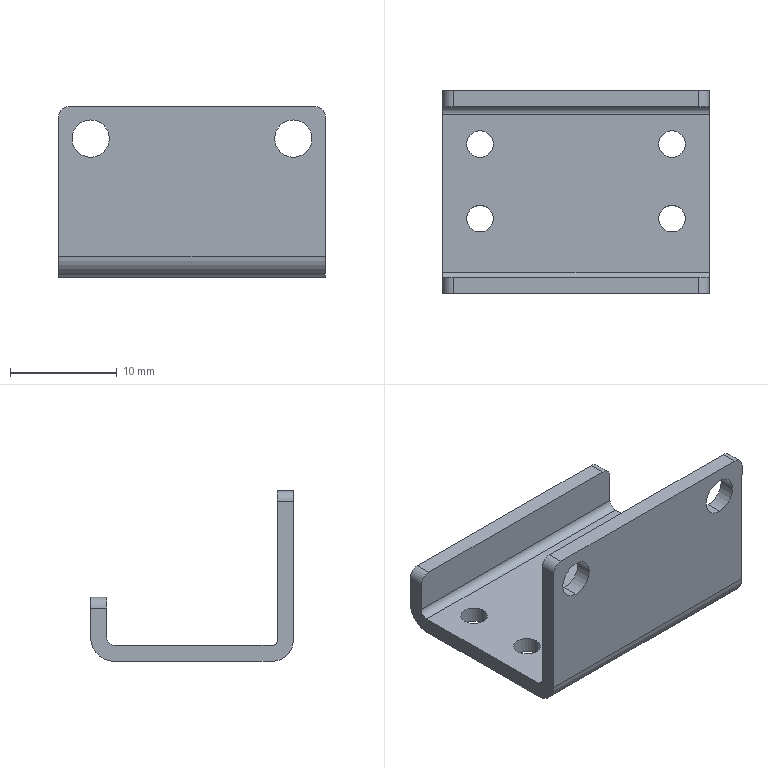Part | SolidWorks | features BaseBody 1 | 1 solid | 30 faces | box 25 x 19 x 16 mm | volume 1321 mm3 | cylinder 20 | plane 10 | commonest cylinder face diameters 2.5 x8 2 x4 3.5 x4 1 x1 1.473 x1 4 x1
STEP:
#1=CARTESIAN_POINT('',(10.25,-2.5,-1.5));
#2=VERTEX_POINT('',#1);
#3=CARTESIAN_POINT('',(7.75,-2.5,-1.5));
#4=VERTEX_POINT('',#3);
#5=CARTESIAN_POINT('',(9.,-2.5,-1.5));
#6=DIRECTION('',(0.,0.,-1.));
#7=DIRECTION('',(1.,0.,0.));
#8=AXIS2_PLACEMENT_3D('',#5,#6,#7);
#9=CIRCLE('',#8,1.25);
#10=EDGE_CURVE('',#2,#4,#9,.T.);
#11=ORIENTED_EDGE('',*,*,#10,.T.);
#12=CARTESIAN_POINT('',(7.75,-2.5,0.));
#13=VERTEX_POINT('',#12);
#14=CARTESIAN_POINT('',(7.75,-2.5,0.));
#15=DIRECTION('',(0.,0.,1.));
#16=VECTOR('',#15,1000.);
#17=LINE('',#14,#16);
#18=EDGE_CURVE('',#4,#13,#17,.T.);
#19=ORIENTED_EDGE('',*,*,#18,.T.);
#20=CARTESIAN_POINT('',(10.25,-2.5,0.));
#21=VERTEX_POINT('',#20);
#22=CARTESIAN_POINT('',(9.,-2.5,0.));
#23=DIRECTION('',(0.,0.,-1.));
#24=DIRECTION('',(1.,0.,0.));
#25=AXIS2_PLACEMENT_3D('',#22,#23,#24);
#26=CIRCLE('',#25,1.25);
#27=EDGE_CURVE('',#21,#13,#26,.T.);
#28=ORIENTED_EDGE('',*,*,#27,.F.);
#29=CARTESIAN_POINT('',(10.25,-2.5,0.));
#30=DIRECTION('',(0.,0.,1.));
#31=VECTOR('',#30,1000.);
#32=LINE('',#29,#31);
#33=EDGE_CURVE('',#2,#21,#32,.T.);
#34=ORIENTED_EDGE('',*,*,#33,.F.);
#35=EDGE_LOOP('',(#11,#19,#28,#34));
#36=FACE_OUTER_BOUND('',#35,.T.);
#37=CARTESIAN_POINT('',(9.,-2.5,0.));
#38=DIRECTION('',(0.,0.,1.));
#39=DIRECTION('',(1.,0.,0.));
#40=AXIS2_PLACEMENT_3D('',#37,#38,#39);
#41=CYLINDRICAL_SURFACE('',#40,1.25);
#42=ADVANCED_FACE('',(#36),#41,.F.);
#43=CARTESIAN_POINT('',(10.25,4.5,-1.5));
#44=VERTEX_POINT('',#43);
#45=CARTESIAN_POINT('',(7.75,4.5,-1.5));
#46=VERTEX_POINT('',#45);
#47=CARTESIAN_POINT('',(9.,4.5,-1.5));
#48=DIRECTION('',(0.,0.,-1.));
#49=DIRECTION('',(1.,0.,0.));
#50=AXIS2_PLACEMENT_3D('',#47,#48,#49);
#51=CIRCLE('',#50,1.25);
#52=EDGE_CURVE('',#44,#46,#51,.T.);
#53=ORIENTED_EDGE('',*,*,#52,.T.);
#54=CARTESIAN_POINT('',(7.75,4.5,0.));
#55=VERTEX_POINT('',#54);
#56=CARTESIAN_POINT('',(7.75,4.5,0.));
#57=DIRECTION('',(0.,0.,1.));
#58=VECTOR('',#57,1000.);
#59=LINE('',#56,#58);
#60=EDGE_CURVE('',#46,#55,#59,.T.);
#61=ORIENTED_EDGE('',*,*,#60,.T.);
#62=CARTESIAN_POINT('',(10.25,4.5,0.));
#63=VERTEX_POINT('',#62);
#64=CARTESIAN_POINT('',(9.,4.5,0.));
#65=DIRECTION('',(0.,0.,-1.));
#66=DIRECTION('',(1.,0.,0.));
#67=AXIS2_PLACEMENT_3D('',#64,#65,#66);
#68=CIRCLE('',#67,1.25);
#69=EDGE_CURVE('',#63,#55,#68,.T.);
#70=ORIENTED_EDGE('',*,*,#69,.F.);
#71=CARTESIAN_POINT('',(10.25,4.5,0.));
#72=DIRECTION('',(0.,0.,1.));
#73=VECTOR('',#72,1000.);
#74=LINE('',#71,#73);
#75=EDGE_CURVE('',#44,#63,#74,.T.);
#76=ORIENTED_EDGE('',*,*,#75,.F.);
#77=EDGE_LOOP('',(#53,#61,#70,#76));
#78=FACE_OUTER_BOUND('',#77,.T.);
#79=CARTESIAN_POINT('',(9.,4.5,0.));
#80=DIRECTION('',(0.,0.,1.));
#81=DIRECTION('',(1.,0.,0.));
#82=AXIS2_PLACEMENT_3D('',#79,#80,#81);
#83=CYLINDRICAL_SURFACE('',#82,1.25);
#84=ADVANCED_FACE('',(#78),#83,.F.);
#85=CARTESIAN_POINT('',(-7.75,-2.5,-1.5));
#86=VERTEX_POINT('',#85);
#87=CARTESIAN_POINT('',(-10.25,-2.5,-1.5));
#88=VERTEX_POINT('',#87);
#89=CARTESIAN_POINT('',(-9.,-2.5,-1.5));
#90=DIRECTION('',(0.,0.,-1.));
#91=DIRECTION('',(1.,0.,0.));
#92=AXIS2_PLACEMENT_3D('',#89,#90,#91);
#93=CIRCLE('',#92,1.25);
#94=EDGE_CURVE('',#86,#88,#93,.T.);
#95=ORIENTED_EDGE('',*,*,#94,.T.);
#96=CARTESIAN_POINT('',(-10.25,-2.5,0.));
#97=VERTEX_POINT('',#96);
#98=CARTESIAN_POINT('',(-10.25,-2.5,0.));
#99=DIRECTION('',(0.,0.,1.));
#100=VECTOR('',#99,1000.);
#101=LINE('',#98,#100);
#102=EDGE_CURVE('',#88,#97,#101,.T.);
#103=ORIENTED_EDGE('',*,*,#102,.T.);
#104=CARTESIAN_POINT('',(-7.75,-2.5,0.));
#105=VERTEX_POINT('',#104);
#106=CARTESIAN_POINT('',(-9.,-2.5,0.));
#107=DIRECTION('',(0.,0.,-1.));
#108=DIRECTION('',(1.,0.,0.));
#109=AXIS2_PLACEMENT_3D('',#106,#107,#108);
#110=CIRCLE('',#109,1.25);
#111=EDGE_CURVE('',#105,#97,#110,.T.);
#112=ORIENTED_EDGE('',*,*,#111,.F.);
#113=CARTESIAN_POINT('',(-7.75,-2.5,0.));
#114=DIRECTION('',(0.,0.,1.));
#115=VECTOR('',#114,1000.);
#116=LINE('',#113,#115);
#117=EDGE_CURVE('',#86,#105,#116,.T.);
#118=ORIENTED_EDGE('',*,*,#117,.F.);
#119=EDGE_LOOP('',(#95,#103,#112,#118));
#120=FACE_OUTER_BOUND('',#119,.T.);
#121=CARTESIAN_POINT('',(-9.,-2.5,0.));
#122=DIRECTION('',(0.,0.,1.));
#123=DIRECTION('',(1.,0.,0.));
#124=AXIS2_PLACEMENT_3D('',#121,#122,#123);
#125=CYLINDRICAL_SURFACE('',#124,1.25);
#126=ADVANCED_FACE('',(#120),#125,.F.);
#127=CARTESIAN_POINT('',(-7.75,4.5,-1.5));
#128=VERTEX_POINT('',#127);
#129=CARTESIAN_POINT('',(-10.25,4.5,-1.5));
#130=VERTEX_POINT('',#129);
#131=CARTESIAN_POINT('',(-9.,4.5,-1.5));
#132=DIRECTION('',(0.,0.,-1.));
#133=DIRECTION('',(1.,0.,0.));
#134=AXIS2_PLACEMENT_3D('',#131,#132,#133);
#135=CIRCLE('',#134,1.25);
#136=EDGE_CURVE('',#128,#130,#135,.T.);
#137=ORIENTED_EDGE('',*,*,#136,.T.);
#138=CARTESIAN_POINT('',(-10.25,4.5,0.));
#139=VERTEX_POINT('',#138);
#140=CARTESIAN_POINT('',(-10.25,4.5,0.));
#141=DIRECTION('',(0.,0.,1.));
#142=VECTOR('',#141,1000.);
#143=LINE('',#140,#142);
#144=EDGE_CURVE('',#130,#139,#143,.T.);
#145=ORIENTED_EDGE('',*,*,#144,.T.);
#146=CARTESIAN_POINT('',(-7.75,4.5,0.));
#147=VERTEX_POINT('',#146);
#148=CARTESIAN_POINT('',(-9.,4.5,0.));
#149=DIRECTION('',(0.,0.,-1.));
#150=DIRECTION('',(1.,0.,0.));
#151=AXIS2_PLACEMENT_3D('',#148,#149,#150);
#152=CIRCLE('',#151,1.25);
#153=EDGE_CURVE('',#147,#139,#152,.T.);
#154=ORIENTED_EDGE('',*,*,#153,.F.);
#155=CARTESIAN_POINT('',(-7.75,4.5,0.));
#156=DIRECTION('',(0.,0.,1.));
#157=VECTOR('',#156,1000.);
#158=LINE('',#155,#157);
#159=EDGE_CURVE('',#128,#147,#158,.T.);
#160=ORIENTED_EDGE('',*,*,#159,.F.);
#161=EDGE_LOOP('',(#137,#145,#154,#160));
#162=FACE_OUTER_BOUND('',#161,.T.);
#163=CARTESIAN_POINT('',(-9.,4.5,0.));
#164=DIRECTION('',(0.,0.,1.));
#165=DIRECTION('',(1.,0.,0.));
#166=AXIS2_PLACEMENT_3D('',#163,#164,#165);
#167=CYLINDRICAL_SURFACE('',#166,1.25);
#168=ADVANCED_FACE('',(#162),#167,.F.);
#169=CARTESIAN_POINT('',(-9.5,-9.5,13.25));
#170=VERTEX_POINT('',#169);
#171=CARTESIAN_POINT('',(-9.5,-9.5,9.75));
#172=VERTEX_POINT('',#171);
#173=CARTESIAN_POINT('',(-9.5,-9.5,11.5));
#174=DIRECTION('',(0.,-1.,0.));
#175=DIRECTION('',(0.,0.,1.));
#176=AXIS2_PLACEMENT_3D('',#173,#174,#175);
#177=CIRCLE('',#176,1.75);
#178=EDGE_CURVE('',#170,#172,#177,.T.);
#179=ORIENTED_EDGE('',*,*,#178,.T.);
#180=CARTESIAN_POINT('',(-9.5,-8.,9.75));
#181=VERTEX_POINT('',#180);
#182=CARTESIAN_POINT('',(-9.5,-9.5,9.75));
#183=DIRECTION('',(0.,1.,0.));
#184=VECTOR('',#183,1000.);
#185=LINE('',#182,#184);
#186=EDGE_CURVE('',#172,#181,#185,.T.);
#187=ORIENTED_EDGE('',*,*,#186,.T.);
#188=CARTESIAN_POINT('',(-9.5,-8.,13.25));
#189=VERTEX_POINT('',#188);
#190=CARTESIAN_POINT('',(-9.5,-8.,11.5));
#191=DIRECTION('',(0.,-1.,0.));
#192=DIRECTION('',(0.,0.,1.));
#193=AXIS2_PLACEMENT_3D('',#190,#191,#192);
#194=CIRCLE('',#193,1.75);
#195=EDGE_CURVE('',#189,#181,#194,.T.);
#196=ORIENTED_EDGE('',*,*,#195,.F.);
#197=CARTESIAN_POINT('',(-9.5,-9.5,13.25));
#198=DIRECTION('',(0.,1.,0.));
#199=VECTOR('',#198,1000.);
#200=LINE('',#197,#199);
#201=EDGE_CURVE('',#170,#189,#200,.T.);
#202=ORIENTED_EDGE('',*,*,#201,.F.);
#203=EDGE_LOOP('',(#179,#187,#196,#202));
#204=FACE_OUTER_BOUND('',#203,.T.);
#205=CARTESIAN_POINT('',(-9.5,-9.5,11.5));
#206=DIRECTION('',(0.,1.,0.));
#207=DIRECTION('',(0.,0.,1.));
#208=AXIS2_PLACEMENT_3D('',#205,#206,#207);
#209=CYLINDRICAL_SURFACE('',#208,1.75);
#210=ADVANCED_FACE('',(#204),#209,.F.);
#211=CARTESIAN_POINT('',(9.5,-9.5,13.25));
#212=VERTEX_POINT('',#211);
#213=CARTESIAN_POINT('',(9.5,-9.5,9.75));
#214=VERTEX_POINT('',#213);
#215=CARTESIAN_POINT('',(9.5,-9.5,11.5));
#216=DIRECTION('',(0.,-1.,0.));
#217=DIRECTION('',(0.,0.,1.));
#218=AXIS2_PLACEMENT_3D('',#215,#216,#217);
#219=CIRCLE('',#218,1.75);
#220=EDGE_CURVE('',#212,#214,#219,.T.);
#221=ORIENTED_EDGE('',*,*,#220,.T.);
#222=CARTESIAN_POINT('',(9.5,-8.,9.75));
#223=VERTEX_POINT('',#222);
#224=CARTESIAN_POINT('',(9.5,-9.5,9.75));
#225=DIRECTION('',(0.,1.,0.));
#226=VECTOR('',#225,1000.);
#227=LINE('',#224,#226);
#228=EDGE_CURVE('',#214,#223,#227,.T.);
#229=ORIENTED_EDGE('',*,*,#228,.T.);
#230=CARTESIAN_POINT('',(9.5,-8.,13.25));
#231=VERTEX_POINT('',#230);
#232=CARTESIAN_POINT('',(9.5,-8.,11.5));
#233=DIRECTION('',(0.,-1.,0.));
#234=DIRECTION('',(0.,0.,1.));
#235=AXIS2_PLACEMENT_3D('',#232,#233,#234);
#236=CIRCLE('',#235,1.75);
#237=EDGE_CURVE('',#231,#223,#236,.T.);
#238=ORIENTED_EDGE('',*,*,#237,.F.);
#239=CARTESIAN_POINT('',(9.5,-9.5,13.25));
#240=DIRECTION('',(0.,1.,0.));
#241=VECTOR('',#240,1000.);
#242=LINE('',#239,#241);
#243=EDGE_CURVE('',#212,#231,#242,.T.);
#244=ORIENTED_EDGE('',*,*,#243,.F.);
#245=EDGE_LOOP('',(#221,#229,#238,#244));
#246=FACE_OUTER_BOUND('',#245,.T.);
#247=CARTESIAN_POINT('',(9.5,-9.5,11.5));
#248=DIRECTION('',(0.,1.,0.));
#249=DIRECTION('',(0.,0.,1.));
#250=AXIS2_PLACEMENT_3D('',#247,#248,#249);
#251=CYLINDRICAL_SURFACE('',#250,1.75);
#252=ADVANCED_FACE('',(#246),#251,.F.);
#253=CARTESIAN_POINT('',(12.5,-7.5,-1.5));
#254=VERTEX_POINT('',#253);
#255=CARTESIAN_POINT('',(12.5,7.263,-1.5));
#256=VERTEX_POINT('',#255);
#257=CARTESIAN_POINT('',(12.5,0.,-1.5));
#258=DIRECTION('',(0.,1.,0.));
#259=VECTOR('',#258,1000.);
#260=LINE('',#257,#259);
#261=EDGE_CURVE('',#254,#256,#260,.T.);
#262=ORIENTED_EDGE('',*,*,#261,.F.);
#263=CARTESIAN_POINT('',(-12.5,-7.5,-1.5));
#264=VERTEX_POINT('',#263);
#265=CARTESIAN_POINT('',(0.,-7.5,-1.5));
#266=DIRECTION('',(1.,0.,0.));
#267=VECTOR('',#266,1000.);
#268=LINE('',#265,#267);
#269=EDGE_CURVE('',#264,#254,#268,.T.);
#270=ORIENTED_EDGE('',*,*,#269,.F.);
#271=CARTESIAN_POINT('',(-12.5,7.263,-1.5));
#272=VERTEX_POINT('',#271);
#273=CARTESIAN_POINT('',(-12.5,0.,-1.5));
#274=DIRECTION('',(0.,-1.,0.));
#275=VECTOR('',#274,1000.);
#276=LINE('',#273,#275);
#277=EDGE_CURVE('',#272,#264,#276,.T.);
#278=ORIENTED_EDGE('',*,*,#277,.F.);
#279=CARTESIAN_POINT('',(0.,7.263,-1.5));
#280=DIRECTION('',(-1.,0.,0.));
#281=VECTOR('',#280,1000.);
#282=LINE('',#279,#281);
#283=EDGE_CURVE('',#256,#272,#282,.T.);
#284=ORIENTED_EDGE('',*,*,#283,.F.);
#285=EDGE_LOOP('',(#262,#270,#278,#284));
#286=FACE_OUTER_BOUND('',#285,.T.);
#287=ORIENTED_EDGE('',*,*,#10,.F.);
#288=CARTESIAN_POINT('',(9.,-2.5,-1.5));
#289=DIRECTION('',(0.,0.,-1.));
#290=DIRECTION('',(1.,0.,0.));
#291=AXIS2_PLACEMENT_3D('',#288,#289,#290);
#292=CIRCLE('',#291,1.25);
#293=EDGE_CURVE('',#4,#2,#292,.T.);
#294=ORIENTED_EDGE('',*,*,#293,.F.);
#295=EDGE_LOOP('',(#287,#294));
#296=FACE_BOUND('',#295,.T.);
#297=ORIENTED_EDGE('',*,*,#52,.F.);
#298=CARTESIAN_POINT('',(9.,4.5,-1.5));
#299=DIRECTION('',(0.,0.,-1.));
#300=DIRECTION('',(1.,0.,0.));
#301=AXIS2_PLACEMENT_3D('',#298,#299,#300);
#302=CIRCLE('',#301,1.25);
#303=EDGE_CURVE('',#46,#44,#302,.T.);
#304=ORIENTED_EDGE('',*,*,#303,.F.);
#305=EDGE_LOOP('',(#297,#304));
#306=FACE_BOUND('',#305,.T.);
#307=ORIENTED_EDGE('',*,*,#94,.F.);
#308=CARTESIAN_POINT('',(-9.,-2.5,-1.5));
#309=DIRECTION('',(0.,0.,-1.));
#310=DIRECTION('',(1.,0.,0.));
#311=AXIS2_PLACEMENT_3D('',#308,#309,#310);
#312=CIRCLE('',#311,1.25);
#313=EDGE_CURVE('',#88,#86,#312,.T.);
#314=ORIENTED_EDGE('',*,*,#313,.F.);
#315=EDGE_LOOP('',(#307,#314));
#316=FACE_BOUND('',#315,.T.);
#317=ORIENTED_EDGE('',*,*,#136,.F.);
#318=CARTESIAN_POINT('',(-9.,4.5,-1.5));
#319=DIRECTION('',(0.,0.,-1.));
#320=DIRECTION('',(1.,0.,0.));
#321=AXIS2_PLACEMENT_3D('',#318,#319,#320);
#322=CIRCLE('',#321,1.25);
#323=EDGE_CURVE('',#130,#128,#322,.T.);
#324=ORIENTED_EDGE('',*,*,#323,.F.);
#325=EDGE_LOOP('',(#317,#324));
#326=FACE_BOUND('',#325,.T.);
#327=CARTESIAN_POINT('',(0.,0.,-1.5));
#328=DIRECTION('',(0.,0.,1.));
#329=DIRECTION('',(1.,0.,0.));
#330=AXIS2_PLACEMENT_3D('',#327,#328,#329);
#331=PLANE('',#330);
#332=ADVANCED_FACE('',(#286,#296,#306,#316,#326),#331,.F.);
#333=CARTESIAN_POINT('',(-12.5,9.5,0.7366));
#334=VERTEX_POINT('',#333);
#335=CARTESIAN_POINT('',(12.5,9.5,0.7366));
#336=VERTEX_POINT('',#335);
#337=CARTESIAN_POINT('',(-12.5,9.5,0.7366));
#338=DIRECTION('',(1.,0.,0.));
#339=VECTOR('',#338,1000.);
#340=LINE('',#337,#339);
#341=EDGE_CURVE('',#334,#336,#340,.T.);
#342=ORIENTED_EDGE('',*,*,#341,.T.);
#343=CARTESIAN_POINT('',(12.5,7.263,0.7366));
#344=DIRECTION('',(-1.,0.,0.));
#345=DIRECTION('',(0.,0.,1.));
#346=AXIS2_PLACEMENT_3D('',#343,#344,#345);
#347=CIRCLE('',#346,2.237);
#348=EDGE_CURVE('',#336,#256,#347,.T.);
#349=ORIENTED_EDGE('',*,*,#348,.T.);
#350=ORIENTED_EDGE('',*,*,#283,.T.);
#351=CARTESIAN_POINT('',(-12.5,7.263,0.7366));
#352=DIRECTION('',(1.,0.,0.));
#353=DIRECTION('',(0.,0.,1.));
#354=AXIS2_PLACEMENT_3D('',#351,#352,#353);
#355=CIRCLE('',#354,2.237);
#356=EDGE_CURVE('',#272,#334,#355,.T.);
#357=ORIENTED_EDGE('',*,*,#356,.T.);
#358=EDGE_LOOP('',(#342,#349,#350,#357));
#359=FACE_OUTER_BOUND('',#358,.T.);
#360=CARTESIAN_POINT('',(-12.5,7.263,0.7366));
#361=DIRECTION('',(-1.,0.,0.));
#362=DIRECTION('',(0.,0.,1.));
#363=AXIS2_PLACEMENT_3D('',#360,#361,#362);
#364=CYLINDRICAL_SURFACE('',#363,2.237);
#365=ADVANCED_FACE('',(#359),#364,.T.);
#366=CARTESIAN_POINT('',(12.5,7.263,0.));
#367=VERTEX_POINT('',#366);
#368=CARTESIAN_POINT('',(12.5,-7.5,0.));
#369=VERTEX_POINT('',#368);
#370=CARTESIAN_POINT('',(12.5,8.,0.));
#371=DIRECTION('',(0.,-1.,0.));
#372=VECTOR('',#371,1000.);
#373=LINE('',#370,#372);
#374=EDGE_CURVE('',#367,#369,#373,.T.);
#375=ORIENTED_EDGE('',*,*,#374,.T.);
#376=CARTESIAN_POINT('',(12.5,-8.,0.5));
#377=VERTEX_POINT('',#376);
#378=CARTESIAN_POINT('',(12.5,-7.5,0.5));
#379=DIRECTION('',(1.,0.,0.));
#380=DIRECTION('',(0.,0.,-1.));
#381=AXIS2_PLACEMENT_3D('',#378,#379,#380);
#382=CIRCLE('',#381,0.5);
#383=EDGE_CURVE('',#377,#369,#382,.T.);
#384=ORIENTED_EDGE('',*,*,#383,.F.);
#385=CARTESIAN_POINT('',(12.5,-8.,13.5));
#386=VERTEX_POINT('',#385);
#387=CARTESIAN_POINT('',(12.5,-8.,14.5));
#388=DIRECTION('',(0.,0.,-1.));
#389=VECTOR('',#388,1000.);
#390=LINE('',#387,#389);
#391=EDGE_CURVE('',#386,#377,#390,.T.);
#392=ORIENTED_EDGE('',*,*,#391,.F.);
#393=CARTESIAN_POINT('',(12.5,-9.5,13.5));
#394=VERTEX_POINT('',#393);
#395=CARTESIAN_POINT('',(12.5,-9.5,13.5));
#396=DIRECTION('',(0.,1.,0.));
#397=VECTOR('',#396,1000.);
#398=LINE('',#395,#397);
#399=EDGE_CURVE('',#394,#386,#398,.T.);
#400=ORIENTED_EDGE('',*,*,#399,.F.);
#401=CARTESIAN_POINT('',(12.5,-9.5,0.5));
#402=VERTEX_POINT('',#401);
#403=CARTESIAN_POINT('',(12.5,-9.5,0.));
#404=DIRECTION('',(0.,0.,-1.));
#405=VECTOR('',#404,1000.);
#406=LINE('',#403,#405);
#407=EDGE_CURVE('',#394,#402,#406,.T.);
#408=ORIENTED_EDGE('',*,*,#407,.T.);
#409=CARTESIAN_POINT('',(12.5,-7.5,0.5));
#410=DIRECTION('',(-1.,0.,0.));
#411=DIRECTION('',(0.,0.,-1.));
#412=AXIS2_PLACEMENT_3D('',#409,#410,#411);
#413=CIRCLE('',#412,2.);
#414=EDGE_CURVE('',#254,#402,#413,.T.);
#415=ORIENTED_EDGE('',*,*,#414,.F.);
#416=ORIENTED_EDGE('',*,*,#261,.T.);
#417=ORIENTED_EDGE('',*,*,#348,.F.);
#418=CARTESIAN_POINT('',(12.5,9.5,3.5));
#419=VERTEX_POINT('',#418);
#420=CARTESIAN_POINT('',(12.5,9.5,0.));
#421=DIRECTION('',(0.,0.,-1.));
#422=VECTOR('',#421,1000.);
#423=LINE('',#420,#422);
#424=EDGE_CURVE('',#419,#336,#423,.T.);
#425=ORIENTED_EDGE('',*,*,#424,.F.);
#426=CARTESIAN_POINT('',(12.5,8.,3.5));
#427=VERTEX_POINT('',#426);
#428=CARTESIAN_POINT('',(12.5,9.5,3.5));
#429=DIRECTION('',(0.,-1.,0.));
#430=VECTOR('',#429,1000.);
#431=LINE('',#428,#430);
#432=EDGE_CURVE('',#419,#427,#431,.T.);
#433=ORIENTED_EDGE('',*,*,#432,.T.);
#434=CARTESIAN_POINT('',(12.5,8.,0.7366));
#435=VERTEX_POINT('',#434);
#436=CARTESIAN_POINT('',(12.5,8.,4.5));
#437=DIRECTION('',(0.,0.,-1.));
#438=VECTOR('',#437,1000.);
#439=LINE('',#436,#438);
#440=EDGE_CURVE('',#427,#435,#439,.T.);
#441=ORIENTED_EDGE('',*,*,#440,.T.);
#442=CARTESIAN_POINT('',(12.5,7.263,0.7366));
#443=DIRECTION('',(-1.,0.,0.));
#444=DIRECTION('',(0.,0.,1.));
#445=AXIS2_PLACEMENT_3D('',#442,#443,#444);
#446=CIRCLE('',#445,0.7366);
#447=EDGE_CURVE('',#435,#367,#446,.T.);
#448=ORIENTED_EDGE('',*,*,#447,.T.);
#449=EDGE_LOOP('',(#375,#384,#392,#400,#408,#415,#416,#417,#425,#433,#441,#448));
#450=FACE_OUTER_BOUND('',#449,.T.);
#451=CARTESIAN_POINT('',(12.5,8.,-1.5));
#452=DIRECTION('',(1.,0.,0.));
#453=DIRECTION('',(0.,1.,0.));
#454=AXIS2_PLACEMENT_3D('',#451,#452,#453);
#455=PLANE('',#454);
#456=ADVANCED_FACE('',(#450),#455,.T.);
#457=CARTESIAN_POINT('',(-12.5,-9.5,0.5));
#458=VERTEX_POINT('',#457);
#459=CARTESIAN_POINT('',(12.5,-9.5,0.5));
#460=DIRECTION('',(-1.,0.,0.));
#461=VECTOR('',#460,1000.);
#462=LINE('',#459,#461);
#463=EDGE_CURVE('',#402,#458,#462,.T.);
#464=ORIENTED_EDGE('',*,*,#463,.T.);
#465=CARTESIAN_POINT('',(-12.5,-7.5,0.5));
#466=DIRECTION('',(1.,0.,0.));
#467=DIRECTION('',(0.,0.,-1.));
#468=AXIS2_PLACEMENT_3D('',#465,#466,#467);
#469=CIRCLE('',#468,2.);
#470=EDGE_CURVE('',#458,#264,#469,.T.);
#471=ORIENTED_EDGE('',*,*,#470,.T.);
#472=ORIENTED_EDGE('',*,*,#269,.T.);
#473=ORIENTED_EDGE('',*,*,#414,.T.);
#474=EDGE_LOOP('',(#464,#471,#472,#473));
#475=FACE_OUTER_BOUND('',#474,.T.);
#476=CARTESIAN_POINT('',(12.5,-7.5,0.5));
#477=DIRECTION('',(1.,0.,0.));
#478=DIRECTION('',(0.,0.,-1.));
#479=AXIS2_PLACEMENT_3D('',#476,#477,#478);
#480=CYLINDRICAL_SURFACE('',#479,2.);
#481=ADVANCED_FACE('',(#475),#480,.T.);
#482=ORIENTED_EDGE('',*,*,#277,.T.);
#483=ORIENTED_EDGE('',*,*,#470,.F.);
#484=CARTESIAN_POINT('',(-12.5,-9.5,13.5));
#485=VERTEX_POINT('',#484);
#486=CARTESIAN_POINT('',(-12.5,-9.5,0.));
#487=DIRECTION('',(0.,0.,1.));
#488=VECTOR('',#487,1000.);
#489=LINE('',#486,#488);
#490=EDGE_CURVE('',#458,#485,#489,.T.);
#491=ORIENTED_EDGE('',*,*,#490,.T.);
#492=CARTESIAN_POINT('',(-12.5,-8.,13.5));
#493=VERTEX_POINT('',#492);
#494=CARTESIAN_POINT('',(-12.5,-9.5,13.5));
#495=DIRECTION('',(0.,-1.,0.));
#496=VECTOR('',#495,1000.);
#497=LINE('',#494,#496);
#498=EDGE_CURVE('',#493,#485,#497,.T.);
#499=ORIENTED_EDGE('',*,*,#498,.F.);
#500=CARTESIAN_POINT('',(-12.5,-8.,0.5));
#501=VERTEX_POINT('',#500);
#502=CARTESIAN_POINT('',(-12.5,-8.,0.));
#503=DIRECTION('',(0.,0.,1.));
#504=VECTOR('',#503,1000.);
#505=LINE('',#502,#504);
#506=EDGE_CURVE('',#501,#493,#505,.T.);
#507=ORIENTED_EDGE('',*,*,#506,.F.);
#508=CARTESIAN_POINT('',(-12.5,-7.5,0.));
#509=VERTEX_POINT('',#508);
#510=CARTESIAN_POINT('',(-12.5,-7.5,0.5));
#511=DIRECTION('',(1.,0.,0.));
#512=DIRECTION('',(0.,0.,-1.));
#513=AXIS2_PLACEMENT_3D('',#510,#511,#512);
#514=CIRCLE('',#513,0.5);
#515=EDGE_CURVE('',#501,#509,#514,.T.);
#516=ORIENTED_EDGE('',*,*,#515,.T.);
#517=CARTESIAN_POINT('',(-12.5,7.263,0.));
#518=VERTEX_POINT('',#517);
#519=CARTESIAN_POINT('',(-12.5,8.,0.));
#520=DIRECTION('',(0.,1.,0.));
#521=VECTOR('',#520,1000.);
#522=LINE('',#519,#521);
#523=EDGE_CURVE('',#509,#518,#522,.T.);
#524=ORIENTED_EDGE('',*,*,#523,.T.);
#525=CARTESIAN_POINT('',(-12.5,8.,0.7366));
#526=VERTEX_POINT('',#525);
#527=CARTESIAN_POINT('',(-12.5,7.263,0.7366));
#528=DIRECTION('',(1.,0.,0.));
#529=DIRECTION('',(0.,0.,1.));
#530=AXIS2_PLACEMENT_3D('',#527,#528,#529);
#531=CIRCLE('',#530,0.7366);
#532=EDGE_CURVE('',#518,#526,#531,.T.);
#533=ORIENTED_EDGE('',*,*,#532,.T.);
#534=CARTESIAN_POINT('',(-12.5,8.,3.5));
#535=VERTEX_POINT('',#534);
#536=CARTESIAN_POINT('',(-12.5,8.,0.));
#537=DIRECTION('',(0.,0.,1.));
#538=VECTOR('',#537,1000.);
#539=LINE('',#536,#538);
#540=EDGE_CURVE('',#526,#535,#539,.T.);
#541=ORIENTED_EDGE('',*,*,#540,.T.);
#542=CARTESIAN_POINT('',(-12.5,9.5,3.5));
#543=VERTEX_POINT('',#542);
#544=CARTESIAN_POINT('',(-12.5,9.5,3.5));
#545=DIRECTION('',(0.,-1.,0.));
#546=VECTOR('',#545,1000.);
#547=LINE('',#544,#546);
#548=EDGE_CURVE('',#543,#535,#547,.T.);
#549=ORIENTED_EDGE('',*,*,#548,.F.);
#550=CARTESIAN_POINT('',(-12.5,9.5,0.));
#551=DIRECTION('',(0.,0.,1.));
#552=VECTOR('',#551,1000.);
#553=LINE('',#550,#552);
#554=EDGE_CURVE('',#334,#543,#553,.T.);
#555=ORIENTED_EDGE('',*,*,#554,.F.);
#556=ORIENTED_EDGE('',*,*,#356,.F.);
#557=EDGE_LOOP('',(#482,#483,#491,#499,#507,#516,#524,#533,#541,#549,#555,#556));
#558=FACE_OUTER_BOUND('',#557,.T.);
#559=CARTESIAN_POINT('',(-12.5,8.,-1.5));
#560=DIRECTION('',(-1.,0.,0.));
#561=DIRECTION('',(0.,-1.,0.));
#562=AXIS2_PLACEMENT_3D('',#559,#560,#561);
#563=PLANE('',#562);
#564=ADVANCED_FACE('',(#558),#563,.T.);
#565=ORIENTED_EDGE('',*,*,#18,.F.);
#566=ORIENTED_EDGE('',*,*,#293,.T.);
#567=ORIENTED_EDGE('',*,*,#33,.T.);
#568=CARTESIAN_POINT('',(9.,-2.5,0.));
#569=DIRECTION('',(0.,0.,-1.));
#570=DIRECTION('',(1.,0.,0.));
#571=AXIS2_PLACEMENT_3D('',#568,#569,#570);
#572=CIRCLE('',#571,1.25);
#573=EDGE_CURVE('',#13,#21,#572,.T.);
#574=ORIENTED_EDGE('',*,*,#573,.F.);
#575=EDGE_LOOP('',(#565,#566,#567,#574));
#576=FACE_OUTER_BOUND('',#575,.T.);
#577=CARTESIAN_POINT('',(9.,-2.5,0.));
#578=DIRECTION('',(0.,0.,1.));
#579=DIRECTION('',(1.,0.,0.));
#580=AXIS2_PLACEMENT_3D('',#577,#578,#579);
#581=CYLINDRICAL_SURFACE('',#580,1.25);
#582=ADVANCED_FACE('',(#576),#581,.F.);
#583=ORIENTED_EDGE('',*,*,#60,.F.);
#584=ORIENTED_EDGE('',*,*,#303,.T.);
#585=ORIENTED_EDGE('',*,*,#75,.T.);
#586=CARTESIAN_POINT('',(9.,4.5,0.));
#587=DIRECTION('',(0.,0.,-1.));
#588=DIRECTION('',(1.,0.,0.));
#589=AXIS2_PLACEMENT_3D('',#586,#587,#588);
#590=CIRCLE('',#589,1.25);
#591=EDGE_CURVE('',#55,#63,#590,.T.);
#592=ORIENTED_EDGE('',*,*,#591,.F.);
#593=EDGE_LOOP('',(#583,#584,#585,#592));
#594=FACE_OUTER_BOUND('',#593,.T.);
#595=CARTESIAN_POINT('',(9.,4.5,0.));
#596=DIRECTION('',(0.,0.,1.));
#597=DIRECTION('',(1.,0.,0.));
#598=AXIS2_PLACEMENT_3D('',#595,#596,#597);
#599=CYLINDRICAL_SURFACE('',#598,1.25);
#600=ADVANCED_FACE('',(#594),#599,.F.);
#601=ORIENTED_EDGE('',*,*,#102,.F.);
#602=ORIENTED_EDGE('',*,*,#313,.T.);
#603=ORIENTED_EDGE('',*,*,#117,.T.);
#604=CARTESIAN_POINT('',(-9.,-2.5,0.));
#605=DIRECTION('',(0.,0.,-1.));
#606=DIRECTION('',(1.,0.,0.));
#607=AXIS2_PLACEMENT_3D('',#604,#605,#606);
#608=CIRCLE('',#607,1.25);
#609=EDGE_CURVE('',#97,#105,#608,.T.);
#610=ORIENTED_EDGE('',*,*,#609,.F.);
#611=EDGE_LOOP('',(#601,#602,#603,#610));
#612=FACE_OUTER_BOUND('',#611,.T.);
#613=CARTESIAN_POINT('',(-9.,-2.5,0.));
#614=DIRECTION('',(0.,0.,1.));
#615=DIRECTION('',(1.,0.,0.));
#616=AXIS2_PLACEMENT_3D('',#613,#614,#615);
#617=CYLINDRICAL_SURFACE('',#616,1.25);
#618=ADVANCED_FACE('',(#612),#617,.F.);
#619=ORIENTED_EDGE('',*,*,#144,.F.);
#620=ORIENTED_EDGE('',*,*,#323,.T.);
#621=ORIENTED_EDGE('',*,*,#159,.T.);
#622=CARTESIAN_POINT('',(-9.,4.5,0.));
#623=DIRECTION('',(0.,0.,-1.));
#624=DIRECTION('',(1.,0.,0.));
#625=AXIS2_PLACEMENT_3D('',#622,#623,#624);
#626=CIRCLE('',#625,1.25);
#627=EDGE_CURVE('',#139,#147,#626,.T.);
#628=ORIENTED_EDGE('',*,*,#627,.F.);
#629=EDGE_LOOP('',(#619,#620,#621,#628));
#630=FACE_OUTER_BOUND('',#629,.T.);
#631=CARTESIAN_POINT('',(-9.,4.5,0.));
#632=DIRECTION('',(0.,0.,1.));
#633=DIRECTION('',(1.,0.,0.));
#634=AXIS2_PLACEMENT_3D('',#631,#632,#633);
#635=CYLINDRICAL_SURFACE('',#634,1.25);
#636=ADVANCED_FACE('',(#630),#635,.F.);
#637=ORIENTED_EDGE('',*,*,#424,.T.);
#638=ORIENTED_EDGE('',*,*,#341,.F.);
#639=ORIENTED_EDGE('',*,*,#554,.T.);
#640=CARTESIAN_POINT('',(-11.5,9.5,4.5));
#641=VERTEX_POINT('',#640);
#642=CARTESIAN_POINT('',(-11.5,9.5,3.5));
#643=DIRECTION('',(0.,1.,0.));
#644=DIRECTION('',(0.,0.,-1.));
#645=AXIS2_PLACEMENT_3D('',#642,#643,#644);
#646=CIRCLE('',#645,1.);
#647=EDGE_CURVE('',#543,#641,#646,.T.);
#648=ORIENTED_EDGE('',*,*,#647,.T.);
#649=CARTESIAN_POINT('',(11.5,9.5,4.5));
#650=VERTEX_POINT('',#649);
#651=CARTESIAN_POINT('',(0.,9.5,4.5));
#652=DIRECTION('',(1.,0.,0.));
#653=VECTOR('',#652,1000.);
#654=LINE('',#651,#653);
#655=EDGE_CURVE('',#641,#650,#654,.T.);
#656=ORIENTED_EDGE('',*,*,#655,.T.);
#657=CARTESIAN_POINT('',(11.5,9.5,3.5));
#658=DIRECTION('',(0.,1.,0.));
#659=DIRECTION('',(0.,0.,-1.));
#660=AXIS2_PLACEMENT_3D('',#657,#658,#659);
#661=CIRCLE('',#660,1.);
#662=EDGE_CURVE('',#650,#419,#661,.T.);
#663=ORIENTED_EDGE('',*,*,#662,.T.);
#664=EDGE_LOOP('',(#637,#638,#639,#648,#656,#663));
#665=FACE_OUTER_BOUND('',#664,.T.);
#666=CARTESIAN_POINT('',(0.,9.5,0.));
#667=DIRECTION('',(0.,1.,0.));
#668=DIRECTION('',(0.,0.,1.));
#669=AXIS2_PLACEMENT_3D('',#666,#667,#668);
#670=PLANE('',#669);
#671=ADVANCED_FACE('',(#665),#670,.T.);
#672=ORIENTED_EDGE('',*,*,#523,.F.);
#673=CARTESIAN_POINT('',(0.,-7.5,0.));
#674=DIRECTION('',(1.,0.,0.));
#675=VECTOR('',#674,1000.);
#676=LINE('',#673,#675);
#677=EDGE_CURVE('',#509,#369,#676,.T.);
#678=ORIENTED_EDGE('',*,*,#677,.T.);
#679=ORIENTED_EDGE('',*,*,#374,.F.);
#680=CARTESIAN_POINT('',(0.,7.263,0.));
#681=DIRECTION('',(-1.,0.,0.));
#682=VECTOR('',#681,1000.);
#683=LINE('',#680,#682);
#684=EDGE_CURVE('',#367,#518,#683,.T.);
#685=ORIENTED_EDGE('',*,*,#684,.T.);
#686=EDGE_LOOP('',(#672,#678,#679,#685));
#687=FACE_OUTER_BOUND('',#686,.T.);
#688=ORIENTED_EDGE('',*,*,#153,.T.);
#689=ORIENTED_EDGE('',*,*,#627,.T.);
#690=EDGE_LOOP('',(#688,#689));
#691=FACE_BOUND('',#690,.T.);
#692=ORIENTED_EDGE('',*,*,#111,.T.);
#693=ORIENTED_EDGE('',*,*,#609,.T.);
#694=EDGE_LOOP('',(#692,#693));
#695=FACE_BOUND('',#694,.T.);
#696=ORIENTED_EDGE('',*,*,#69,.T.);
#697=ORIENTED_EDGE('',*,*,#591,.T.);
#698=EDGE_LOOP('',(#696,#697));
#699=FACE_BOUND('',#698,.T.);
#700=ORIENTED_EDGE('',*,*,#27,.T.);
#701=ORIENTED_EDGE('',*,*,#573,.T.);
#702=EDGE_LOOP('',(#700,#701));
#703=FACE_BOUND('',#702,.T.);
#704=CARTESIAN_POINT('',(0.,0.,0.));
#705=DIRECTION('',(0.,0.,1.));
#706=DIRECTION('',(1.,0.,0.));
#707=AXIS2_PLACEMENT_3D('',#704,#705,#706);
#708=PLANE('',#707);
#709=ADVANCED_FACE('',(#687,#691,#695,#699,#703),#708,.T.);
#710=CARTESIAN_POINT('',(11.5,-9.5,14.5));
#711=VERTEX_POINT('',#710);
#712=CARTESIAN_POINT('',(11.5,-9.5,13.5));
#713=DIRECTION('',(0.,1.,0.));
#714=DIRECTION('',(0.,0.,1.));
#715=AXIS2_PLACEMENT_3D('',#712,#713,#714);
#716=CIRCLE('',#715,1.);
#717=EDGE_CURVE('',#711,#394,#716,.T.);
#718=ORIENTED_EDGE('',*,*,#717,.F.);
#719=CARTESIAN_POINT('',(-11.5,-9.5,14.5));
#720=VERTEX_POINT('',#719);
#721=CARTESIAN_POINT('',(0.,-9.5,14.5));
#722=DIRECTION('',(1.,0.,0.));
#723=VECTOR('',#722,1000.);
#724=LINE('',#721,#723);
#725=EDGE_CURVE('',#720,#711,#724,.T.);
#726=ORIENTED_EDGE('',*,*,#725,.F.);
#727=CARTESIAN_POINT('',(-11.5,-9.5,13.5));
#728=DIRECTION('',(0.,1.,0.));
#729=DIRECTION('',(0.,0.,1.));
#730=AXIS2_PLACEMENT_3D('',#727,#728,#729);
#731=CIRCLE('',#730,1.);
#732=EDGE_CURVE('',#485,#720,#731,.T.);
#733=ORIENTED_EDGE('',*,*,#732,.F.);
#734=ORIENTED_EDGE('',*,*,#490,.F.);
#735=ORIENTED_EDGE('',*,*,#463,.F.);
#736=ORIENTED_EDGE('',*,*,#407,.F.);
#737=EDGE_LOOP('',(#718,#726,#733,#734,#735,#736));
#738=FACE_OUTER_BOUND('',#737,.T.);
#739=ORIENTED_EDGE('',*,*,#178,.F.);
#740=CARTESIAN_POINT('',(-9.5,-9.5,11.5));
#741=DIRECTION('',(0.,-1.,0.));
#742=DIRECTION('',(0.,0.,1.));
#743=AXIS2_PLACEMENT_3D('',#740,#741,#742);
#744=CIRCLE('',#743,1.75);
#745=EDGE_CURVE('',#172,#170,#744,.T.);
#746=ORIENTED_EDGE('',*,*,#745,.F.);
#747=EDGE_LOOP('',(#739,#746));
#748=FACE_BOUND('',#747,.T.);
#749=ORIENTED_EDGE('',*,*,#220,.F.);
#750=CARTESIAN_POINT('',(9.5,-9.5,11.5));
#751=DIRECTION('',(0.,-1.,0.));
#752=DIRECTION('',(0.,0.,1.));
#753=AXIS2_PLACEMENT_3D('',#750,#751,#752);
#754=CIRCLE('',#753,1.75);
#755=EDGE_CURVE('',#214,#212,#754,.T.);
#756=ORIENTED_EDGE('',*,*,#755,.F.);
#757=EDGE_LOOP('',(#749,#756));
#758=FACE_BOUND('',#757,.T.);
#759=CARTESIAN_POINT('',(0.,-9.5,0.));
#760=DIRECTION('',(0.,1.,0.));
#761=DIRECTION('',(0.,0.,1.));
#762=AXIS2_PLACEMENT_3D('',#759,#760,#761);
#763=PLANE('',#762);
#764=ADVANCED_FACE('',(#738,#748,#758),#763,.F.);
#765=CARTESIAN_POINT('',(11.5,8.,4.5));
#766=VERTEX_POINT('',#765);
#767=CARTESIAN_POINT('',(11.5,8.,3.5));
#768=DIRECTION('',(0.,1.,0.));
#769=DIRECTION('',(0.,0.,-1.));
#770=AXIS2_PLACEMENT_3D('',#767,#768,#769);
#771=CIRCLE('',#770,1.);
#772=EDGE_CURVE('',#766,#427,#771,.T.);
#773=ORIENTED_EDGE('',*,*,#772,.T.);
#774=ORIENTED_EDGE('',*,*,#432,.F.);
#775=ORIENTED_EDGE('',*,*,#662,.F.);
#776=CARTESIAN_POINT('',(11.5,9.5,4.5));
#777=DIRECTION('',(0.,-1.,0.));
#778=VECTOR('',#777,1000.);
#779=LINE('',#776,#778);
#780=EDGE_CURVE('',#650,#766,#779,.T.);
#781=ORIENTED_EDGE('',*,*,#780,.T.);
#782=EDGE_LOOP('',(#773,#774,#775,#781));
#783=FACE_OUTER_BOUND('',#782,.T.);
#784=CARTESIAN_POINT('',(11.5,9.5,3.5));
#785=DIRECTION('',(0.,-1.,0.));
#786=DIRECTION('',(0.,0.,-1.));
#787=AXIS2_PLACEMENT_3D('',#784,#785,#786);
#788=CYLINDRICAL_SURFACE('',#787,1.);
#789=ADVANCED_FACE('',(#783),#788,.T.);
#790=CARTESIAN_POINT('',(-11.5,8.,4.5));
#791=VERTEX_POINT('',#790);
#792=CARTESIAN_POINT('',(-12.5,8.,4.5));
#793=DIRECTION('',(1.,0.,0.));
#794=VECTOR('',#793,1000.);
#795=LINE('',#792,#794);
#796=EDGE_CURVE('',#791,#766,#795,.T.);
#797=ORIENTED_EDGE('',*,*,#796,.T.);
#798=ORIENTED_EDGE('',*,*,#780,.F.);
#799=ORIENTED_EDGE('',*,*,#655,.F.);
#800=CARTESIAN_POINT('',(-11.5,9.5,4.5));
#801=DIRECTION('',(0.,-1.,0.));
#802=VECTOR('',#801,1000.);
#803=LINE('',#800,#802);
#804=EDGE_CURVE('',#641,#791,#803,.T.);
#805=ORIENTED_EDGE('',*,*,#804,.T.);
#806=EDGE_LOOP('',(#797,#798,#799,#805));
#807=FACE_OUTER_BOUND('',#806,.T.);
#808=CARTESIAN_POINT('',(-12.5,9.5,4.5));
#809=DIRECTION('',(0.,0.,1.));
#810=DIRECTION('',(0.,-1.,0.));
#811=AXIS2_PLACEMENT_3D('',#808,#809,#810);
#812=PLANE('',#811);
#813=ADVANCED_FACE('',(#807),#812,.T.);
#814=CARTESIAN_POINT('',(-11.5,8.,3.5));
#815=DIRECTION('',(0.,1.,0.));
#816=DIRECTION('',(0.,0.,-1.));
#817=AXIS2_PLACEMENT_3D('',#814,#815,#816);
#818=CIRCLE('',#817,1.);
#819=EDGE_CURVE('',#535,#791,#818,.T.);
#820=ORIENTED_EDGE('',*,*,#819,.T.);
#821=ORIENTED_EDGE('',*,*,#804,.F.);
#822=ORIENTED_EDGE('',*,*,#647,.F.);
#823=ORIENTED_EDGE('',*,*,#548,.T.);
#824=EDGE_LOOP('',(#820,#821,#822,#823));
#825=FACE_OUTER_BOUND('',#824,.T.);
#826=CARTESIAN_POINT('',(-11.5,9.5,3.5));
#827=DIRECTION('',(0.,-1.,0.));
#828=DIRECTION('',(0.,0.,-1.));
#829=AXIS2_PLACEMENT_3D('',#826,#827,#828);
#830=CYLINDRICAL_SURFACE('',#829,1.);
#831=ADVANCED_FACE('',(#825),#830,.T.);
#832=ORIENTED_EDGE('',*,*,#515,.F.);
#833=CARTESIAN_POINT('',(12.5,-8.,0.5));
#834=DIRECTION('',(-1.,0.,0.));
#835=VECTOR('',#834,1000.);
#836=LINE('',#833,#835);
#837=EDGE_CURVE('',#377,#501,#836,.T.);
#838=ORIENTED_EDGE('',*,*,#837,.F.);
#839=ORIENTED_EDGE('',*,*,#383,.T.);
#840=ORIENTED_EDGE('',*,*,#677,.F.);
#841=EDGE_LOOP('',(#832,#838,#839,#840));
#842=FACE_OUTER_BOUND('',#841,.T.);
#843=CARTESIAN_POINT('',(12.5,-7.5,0.5));
#844=DIRECTION('',(1.,0.,0.));
#845=DIRECTION('',(0.,0.,-1.));
#846=AXIS2_PLACEMENT_3D('',#843,#844,#845);
#847=CYLINDRICAL_SURFACE('',#846,0.5);
#848=ADVANCED_FACE('',(#842),#847,.F.);
#849=ORIENTED_EDGE('',*,*,#447,.F.);
#850=CARTESIAN_POINT('',(-12.5,8.,0.7366));
#851=DIRECTION('',(1.,0.,0.));
#852=VECTOR('',#851,1000.);
#853=LINE('',#850,#852);
#854=EDGE_CURVE('',#526,#435,#853,.T.);
#855=ORIENTED_EDGE('',*,*,#854,.F.);
#856=ORIENTED_EDGE('',*,*,#532,.F.);
#857=ORIENTED_EDGE('',*,*,#684,.F.);
#858=EDGE_LOOP('',(#849,#855,#856,#857));
#859=FACE_OUTER_BOUND('',#858,.T.);
#860=CARTESIAN_POINT('',(-12.5,7.263,0.7366));
#861=DIRECTION('',(-1.,0.,0.));
#862=DIRECTION('',(0.,0.,1.));
#863=AXIS2_PLACEMENT_3D('',#860,#861,#862);
#864=CYLINDRICAL_SURFACE('',#863,0.7366);
#865=ADVANCED_FACE('',(#859),#864,.F.);
#866=CARTESIAN_POINT('',(11.5,-8.,14.5));
#867=VERTEX_POINT('',#866);
#868=CARTESIAN_POINT('',(11.5,-8.,13.5));
#869=DIRECTION('',(0.,-1.,0.));
#870=DIRECTION('',(0.,0.,1.));
#871=AXIS2_PLACEMENT_3D('',#868,#869,#870);
#872=CIRCLE('',#871,1.);
#873=EDGE_CURVE('',#386,#867,#872,.T.);
#874=ORIENTED_EDGE('',*,*,#873,.T.);
#875=CARTESIAN_POINT('',(11.5,-9.5,14.5));
#876=DIRECTION('',(0.,-1.,0.));
#877=VECTOR('',#876,1000.);
#878=LINE('',#875,#877);
#879=EDGE_CURVE('',#867,#711,#878,.T.);
#880=ORIENTED_EDGE('',*,*,#879,.T.);
#881=ORIENTED_EDGE('',*,*,#717,.T.);
#882=ORIENTED_EDGE('',*,*,#399,.T.);
#883=EDGE_LOOP('',(#874,#880,#881,#882));
#884=FACE_OUTER_BOUND('',#883,.T.);
#885=CARTESIAN_POINT('',(11.5,-9.5,13.5));
#886=DIRECTION('',(0.,1.,0.));
#887=DIRECTION('',(0.,0.,1.));
#888=AXIS2_PLACEMENT_3D('',#885,#886,#887);
#889=CYLINDRICAL_SURFACE('',#888,1.);
#890=ADVANCED_FACE('',(#884),#889,.T.);
#891=ORIENTED_EDGE('',*,*,#879,.F.);
#892=CARTESIAN_POINT('',(-11.5,-8.,14.5));
#893=VERTEX_POINT('',#892);
#894=CARTESIAN_POINT('',(-12.5,-8.,14.5));
#895=DIRECTION('',(1.,0.,0.));
#896=VECTOR('',#895,1000.);
#897=LINE('',#894,#896);
#898=EDGE_CURVE('',#893,#867,#897,.T.);
#899=ORIENTED_EDGE('',*,*,#898,.F.);
#900=CARTESIAN_POINT('',(-11.5,-9.5,14.5));
#901=DIRECTION('',(0.,1.,0.));
#902=VECTOR('',#901,1000.);
#903=LINE('',#900,#902);
#904=EDGE_CURVE('',#720,#893,#903,.T.);
#905=ORIENTED_EDGE('',*,*,#904,.F.);
#906=ORIENTED_EDGE('',*,*,#725,.T.);
#907=EDGE_LOOP('',(#891,#899,#905,#906));
#908=FACE_OUTER_BOUND('',#907,.T.);
#909=CARTESIAN_POINT('',(-12.5,-9.5,14.5));
#910=DIRECTION('',(0.,0.,-1.));
#911=DIRECTION('',(0.,1.,0.));
#912=AXIS2_PLACEMENT_3D('',#909,#910,#911);
#913=PLANE('',#912);
#914=ADVANCED_FACE('',(#908),#913,.F.);
#915=CARTESIAN_POINT('',(-11.5,-8.,13.5));
#916=DIRECTION('',(0.,-1.,0.));
#917=DIRECTION('',(0.,0.,1.));
#918=AXIS2_PLACEMENT_3D('',#915,#916,#917);
#919=CIRCLE('',#918,1.);
#920=EDGE_CURVE('',#893,#493,#919,.T.);
#921=ORIENTED_EDGE('',*,*,#920,.T.);
#922=ORIENTED_EDGE('',*,*,#498,.T.);
#923=ORIENTED_EDGE('',*,*,#732,.T.);
#924=ORIENTED_EDGE('',*,*,#904,.T.);
#925=EDGE_LOOP('',(#921,#922,#923,#924));
#926=FACE_OUTER_BOUND('',#925,.T.);
#927=CARTESIAN_POINT('',(-11.5,-9.5,13.5));
#928=DIRECTION('',(0.,1.,0.));
#929=DIRECTION('',(0.,0.,1.));
#930=AXIS2_PLACEMENT_3D('',#927,#928,#929);
#931=CYLINDRICAL_SURFACE('',#930,1.);
#932=ADVANCED_FACE('',(#926),#931,.T.);
#933=ORIENTED_EDGE('',*,*,#186,.F.);
#934=ORIENTED_EDGE('',*,*,#745,.T.);
#935=ORIENTED_EDGE('',*,*,#201,.T.);
#936=CARTESIAN_POINT('',(-9.5,-8.,11.5));
#937=DIRECTION('',(0.,-1.,0.));
#938=DIRECTION('',(0.,0.,1.));
#939=AXIS2_PLACEMENT_3D('',#936,#937,#938);
#940=CIRCLE('',#939,1.75);
#941=EDGE_CURVE('',#181,#189,#940,.T.);
#942=ORIENTED_EDGE('',*,*,#941,.F.);
#943=EDGE_LOOP('',(#933,#934,#935,#942));
#944=FACE_OUTER_BOUND('',#943,.T.);
#945=CARTESIAN_POINT('',(-9.5,-9.5,11.5));
#946=DIRECTION('',(0.,1.,0.));
#947=DIRECTION('',(0.,0.,1.));
#948=AXIS2_PLACEMENT_3D('',#945,#946,#947);
#949=CYLINDRICAL_SURFACE('',#948,1.75);
#950=ADVANCED_FACE('',(#944),#949,.F.);
#951=ORIENTED_EDGE('',*,*,#228,.F.);
#952=ORIENTED_EDGE('',*,*,#755,.T.);
#953=ORIENTED_EDGE('',*,*,#243,.T.);
#954=CARTESIAN_POINT('',(9.5,-8.,11.5));
#955=DIRECTION('',(0.,-1.,0.));
#956=DIRECTION('',(0.,0.,1.));
#957=AXIS2_PLACEMENT_3D('',#954,#955,#956);
#958=CIRCLE('',#957,1.75);
#959=EDGE_CURVE('',#223,#231,#958,.T.);
#960=ORIENTED_EDGE('',*,*,#959,.F.);
#961=EDGE_LOOP('',(#951,#952,#953,#960));
#962=FACE_OUTER_BOUND('',#961,.T.);
#963=CARTESIAN_POINT('',(9.5,-9.5,11.5));
#964=DIRECTION('',(0.,1.,0.));
#965=DIRECTION('',(0.,0.,1.));
#966=AXIS2_PLACEMENT_3D('',#963,#964,#965);
#967=CYLINDRICAL_SURFACE('',#966,1.75);
#968=ADVANCED_FACE('',(#962),#967,.F.);
#969=ORIENTED_EDGE('',*,*,#819,.F.);
#970=ORIENTED_EDGE('',*,*,#540,.F.);
#971=ORIENTED_EDGE('',*,*,#854,.T.);
#972=ORIENTED_EDGE('',*,*,#440,.F.);
#973=ORIENTED_EDGE('',*,*,#772,.F.);
#974=ORIENTED_EDGE('',*,*,#796,.F.);
#975=EDGE_LOOP('',(#969,#970,#971,#972,#973,#974));
#976=FACE_OUTER_BOUND('',#975,.T.);
#977=CARTESIAN_POINT('',(0.,8.,0.));
#978=DIRECTION('',(0.,1.,0.));
#979=DIRECTION('',(0.,0.,1.));
#980=AXIS2_PLACEMENT_3D('',#977,#978,#979);
#981=PLANE('',#980);
#982=ADVANCED_FACE('',(#976),#981,.F.);
#983=ORIENTED_EDGE('',*,*,#506,.T.);
#984=ORIENTED_EDGE('',*,*,#920,.F.);
#985=ORIENTED_EDGE('',*,*,#898,.T.);
#986=ORIENTED_EDGE('',*,*,#873,.F.);
#987=ORIENTED_EDGE('',*,*,#391,.T.);
#988=ORIENTED_EDGE('',*,*,#837,.T.);
#989=EDGE_LOOP('',(#983,#984,#985,#986,#987,#988));
#990=FACE_OUTER_BOUND('',#989,.T.);
#991=ORIENTED_EDGE('',*,*,#195,.T.);
#992=ORIENTED_EDGE('',*,*,#941,.T.);
#993=EDGE_LOOP('',(#991,#992));
#994=FACE_BOUND('',#993,.T.);
#995=ORIENTED_EDGE('',*,*,#237,.T.);
#996=ORIENTED_EDGE('',*,*,#959,.T.);
#997=EDGE_LOOP('',(#995,#996));
#998=FACE_BOUND('',#997,.T.);
#999=CARTESIAN_POINT('',(0.,-8.,0.));
#1000=DIRECTION('',(0.,1.,0.));
#1001=DIRECTION('',(0.,0.,1.));
#1002=AXIS2_PLACEMENT_3D('',#999,#1000,#1001);
#1003=PLANE('',#1002);
#1004=ADVANCED_FACE('',(#990,#994,#998),#1003,.T.);
#1005=CLOSED_SHELL('',(#42,#84,#126,#168,#210,#252,#332,#365,#456,#481,#564,#582,#600,#618,#636,#671,#709,#764,#789,#813,#831,#848,#865,#890,#914,#932,#950,#968,#982,#1004));
#1006=MANIFOLD_SOLID_BREP('',#1005);
#1007=CARTESIAN_POINT('',(0.,0.,0.));
#1008=DIRECTION('',(0.,0.,1.));
#1009=DIRECTION('',(1.,0.,0.));
#1010=AXIS2_PLACEMENT_3D('',#1007,#1008,#1009);
#1011=(LENGTH_UNIT()NAMED_UNIT(*)SI_UNIT(.MILLI.,.METRE.));
#1012=UNCERTAINTY_MEASURE_WITH_UNIT(LENGTH_MEASURE(0.00001),#1011,'','');
#1013=(NAMED_UNIT(*)PLANE_ANGLE_UNIT()SI_UNIT($,.RADIAN.));
#1014=(NAMED_UNIT(*)SI_UNIT($,.STERADIAN.)SOLID_ANGLE_UNIT());
#1015=(GEOMETRIC_REPRESENTATION_CONTEXT(3)GLOBAL_UNCERTAINTY_ASSIGNED_CONTEXT((#1012))GLOBAL_UNIT_ASSIGNED_CONTEXT((#1011,#1013,#1014))REPRESENTATION_CONTEXT('',''));
#1016=ADVANCED_BREP_SHAPE_REPRESENTATION('',(#1006,#1010),#1015);